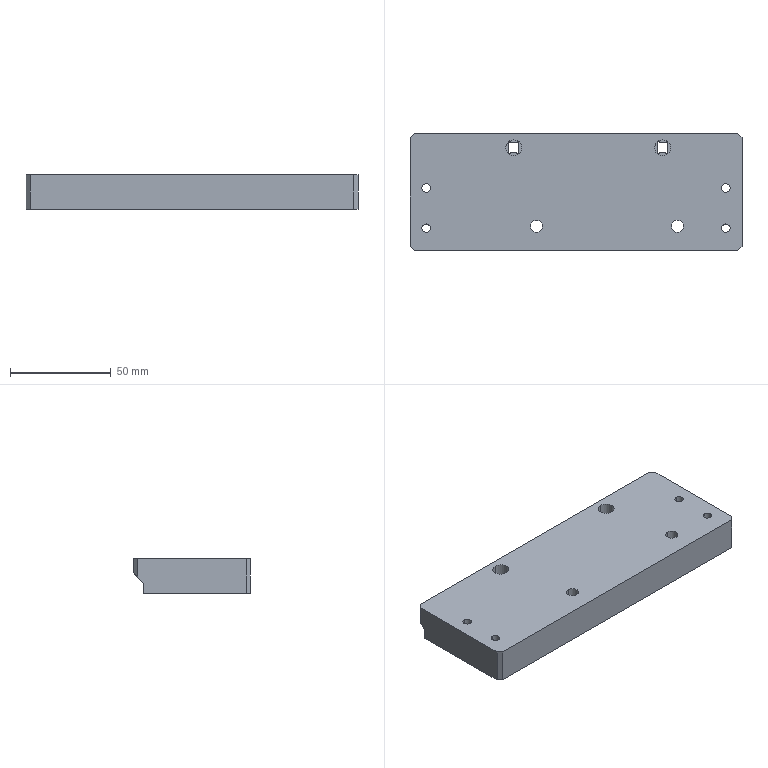NC program | NX | posted with a generic post | part box 165 x 58 x 17 mm
Whole program:
N10 G17 G21 G94 G90
(FLOOR_WALL_COPY , TOOL : D80)
N12 T19 M6
N14 G54
N16 G17 G0 G90 X-125.5 Y0. S6500 M3
N18 G43 Z30. H19
N20 Z5.
N22 G94 G1 Z2. F1500.
N24 X-122.5
N26 X122.5
N28 X125.5
N30 Z5.
N32 G0 Z30.
N34 X-125.5
N36 Z4.
N38 G1 Z1.
N40 X-122.5
N42 X122.5
N44 X125.5
N46 Z4.
N48 G0 Z30.
N50 X-125.5
N52 Z3.
N54 G1 Z0.
N56 X-122.5
N58 X122.5
N60 X125.5
N62 Z3.
N64 G0 Z30.
N66 M5
(HOLE_MILLING_1_COPY , TOOL : D4)
N68 T11 M6
N70 G54
N72 G17 G0 G90 X-30.955 Y21.93 S9500 M3
N74 G43 Z30. H11
N76 Z0.5
N78 G94 G3 X-29.955 Y20.93 R1. F1800.
N80 X-28.955 Y21.93 R1.
N82 X-28.955 Y21.93 Z0.1 I-2. J0.
N84 X-28.955 Y21.93 Z-0.3 I-2. J0.
N86 X-28.955 Y21.93 Z-0.7 I-2. J0.
N88 X-28.955 Y21.93 Z-1.1 I-2. J0.
N90 X-28.955 Y21.93 Z-1.5 I-2. J0.
N92 X-28.955 Y21.93 Z-1.9 I-2. J0.
N94 X-28.955 Y21.93 Z-2.3 I-2. J0.
N96 X-28.955 Y21.93 Z-2.7 I-2. J0.
N98 X-28.955 Y21.93 Z-3.1 I-2. J0.
N100 X-28.955 Y21.93 Z-3.5 I-2. J0.
N102 X-28.955 Y21.93 Z-3.9 I-2. J0.
N104 X-28.955 Y21.93 Z-4.3 I-2. J0.
N106 X-28.955 Y21.93 Z-4.7 I-2. J0.
N108 X-28.955 Y21.93 Z-5.1 I-2. J0.
N110 X-28.955 Y21.93 Z-5.5 I-2. J0.
N112 X-28.955 Y21.93 Z-5.9 I-2. J0.
N114 X-28.955 Y21.93 Z-6.3 I-2. J0.
N116 X-28.955 Y21.93 Z-6.7 I-2. J0.
N118 X-28.955 Y21.93 Z-7.1 I-2. J0.
N120 X-28.955 Y21.93 Z-7.5 I-2. J0.
N122 X-28.955 Y21.93 Z-7.9 I-2. J0.
N124 X-28.955 Y21.93 Z-8.3 I-2. J0.
N126 X-28.955 Y21.93 Z-8.7 I-2. J0.
N128 X-30.955 Y19.93 Z-9. R-2.
N130 X-28.955 Y21.93 R2.
N132 X-30.955 Y19.93 R-2.
N134 X-29.955 Y20.93 R1.
N136 X-30.955 Y21.93 R1.
N138 G0 Z30.
N140 X43.045
N142 Z0.5
N144 G3 X44.045 Y20.93 R1.
N146 X45.045 Y21.93 R1.
N148 X45.045 Y21.93 Z0.1 I-2. J0.
N150 X45.045 Y21.93 Z-0.3 I-2. J0.
N152 X45.045 Y21.93 Z-0.7 I-2. J0.
N154 X45.045 Y21.93 Z-1.1 I-2. J0.
N156 X45.045 Y21.93 Z-1.5 I-2. J0.
N158 X45.045 Y21.93 Z-1.9 I-2. J0.
N160 X45.045 Y21.93 Z-2.3 I-2. J0.
N162 X45.045 Y21.93 Z-2.7 I-2. J0.
N164 X45.045 Y21.93 Z-3.1 I-2. J0.
N166 X45.045 Y21.93 Z-3.5 I-2. J0.
N168 X45.045 Y21.93 Z-3.9 I-2. J0.
N170 X45.045 Y21.93 Z-4.3 I-2. J0.
N172 X45.045 Y21.93 Z-4.7 I-2. J0.
N174 X45.045 Y21.93 Z-5.1 I-2. J0.
N176 X45.045 Y21.93 Z-5.5 I-2. J0.
N178 X45.045 Y21.93 Z-5.9 I-2. J0.
N180 X45.045 Y21.93 Z-6.3 I-2. J0.
N182 X45.045 Y21.93 Z-6.7 I-2. J0.
N184 X45.045 Y21.93 Z-7.1 I-2. J0.
N186 X45.045 Y21.93 Z-7.5 I-2. J0.
N188 X45.045 Y21.93 Z-7.9 I-2. J0.
N190 X45.045 Y21.93 Z-8.3 I-2. J0.
N192 X45.045 Y21.93 Z-8.7 I-2. J0.
N194 X43.045 Y19.93 Z-9. R-2.
N196 X45.045 Y21.93 R2.
N198 X43.045 Y19.93 R-2.
N200 X44.045 Y20.93 R1.
N202 X43.045 Y21.93 R1.
N204 G0 Z30.
N206 M5
(PLANAR_MILL_COPY_COPY_COPY , TOOL : D6A45)
N208 T01 M6
N210 G54
N212 G17 G0 G90 X49.514 Y-18.6 S9500 M3
N214 G43 Z30. H1
N216 Z0.5
N218 G94 G1 Z-1. F1250.
N220 G3 X50.38 Y-19.1 R1.
N222 X52.48 Y-17. R2.1
N224 X50.38 Y-19.1 R-2.1
N226 X51.246 Y-18.6 R1.
N228 G1 Z0.5
N230 G0 Z30.
N232 X75.2 Y-18.866
N234 Z0.5
N236 G1 Z-1.
N238 G3 X75.7 Y-18. R1.
N240 X74.5 Y-16.8 R1.2
N242 X75.7 Y-18. R-1.2
N244 X75.2 Y-17.134 R1.
N246 G1 Z0.5
N248 G0 Z30.
N250 Y1.134
N252 Z0.5
N254 G1 Z-1.
N256 G3 X75.7 Y2. R1.
N258 X74.5 Y3.2 R1.2
N260 X75.7 Y2. R-1.2
N262 X75.2 Y2.866 R1.
N264 G1 Z0.5
N266 G0 Z30.
N268 X43.911 Y24.53
N270 Z0.5
N272 G1 Z-1.
N274 G3 X43.045 Y25.03 R1.
N276 X39.945 Y21.93 R3.1
N278 X43.045 Y25.03 R-3.1
N280 X42.179 Y24.53 R1.
N282 G1 Z0.5
N284 G0 Z30.
N286 X-0.866 Y30.4
N288 Z0.5
N290 G1 Z-1.
N292 G3 X0. Y29.9 R1.
N294 G1 X80.5
N296 G2 X81.136 Y29.636 R0.9
N298 G1 X83.136 Y27.636
N300 G2 X83.4 Y27. R0.9
N302 G1 Y-27.
N304 G2 X83.136 Y-27.636 R0.9
N306 G1 X81.136 Y-29.636
N308 G2 X80.5 Y-29.9 R0.9
N310 G1 X-80.5
N312 G2 X-81.136 Y-29.636 R0.9
N314 G1 X-83.136 Y-27.636
N316 G2 X-83.4 Y-27. R0.9
N318 G1 Y27.
N320 G2 X-83.136 Y27.636 R0.9
N322 G1 X-81.136 Y29.636
N324 G2 X-80.5 Y29.9 R0.9
N326 G1 X0.
N328 G3 X0.866 Y30.4 R1.
N330 G1 Z0.5
N332 G0 Z30.
N334 X-20.486 Y-18.6
N336 Z0.5
N338 G1 Z-1.
N340 G3 X-19.62 Y-19.1 R1.
N342 X-17.52 Y-17. R2.1
N344 X-19.62 Y-19.1 R-2.1
N346 X-18.754 Y-18.6 R1.
N348 G1 Z0.5
N350 G0 Z30.
N352 X-30.089 Y24.53
N354 Z0.5
N356 G1 Z-1.
N358 G3 X-30.955 Y25.03 R1.
N360 X-34.055 Y21.93 R3.1
N362 X-30.955 Y25.03 R-3.1
N364 X-31.821 Y24.53 R1.
N366 G1 Z0.5
N368 G0 Z30.
N370 X-75.2 Y2.866
N372 Z0.5
N374 G1 Z-1.
N376 G3 X-75.7 Y2. R1.
N378 X-74.5 Y0.8 R1.2
N380 X-75.7 Y2. R-1.2
N382 X-75.2 Y1.134 R1.
N384 G1 Z0.5
N386 G0 Z30.
N388 Y-17.134
N390 Z0.5
N392 G1 Z-1.
N394 G3 X-75.7 Y-18. R1.
N396 X-74.5 Y-19.2 R1.2
N398 X-75.7 Y-18. R-1.2
N400 X-75.2 Y-18.866 R1.
N402 G1 Z0.5
N404 G0 Z30.
N406 M5
N408 M2